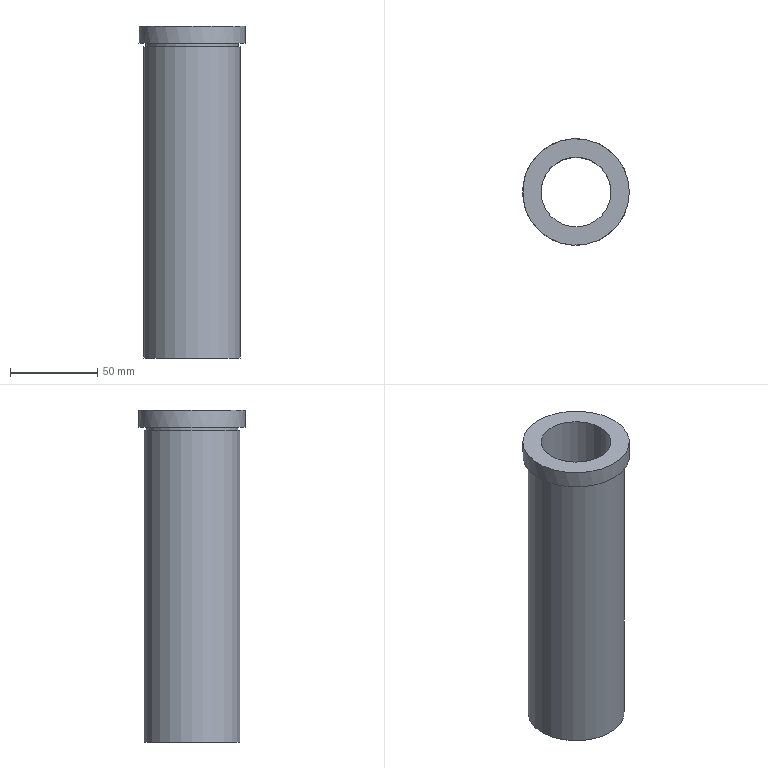Part | STEP file | 车灯-后视镜_id62_x_t | 1 solid | 8 faces | box 61 x 61 x 190 mm | volume 217774 mm3 | plane 4 | cylinder 4 | commonest cylinder face diameters 40 x1 53 x1 55 x1 61 x1
STEP:
#1=CARTESIAN_POINT('',(176.5,-230.,180.5));
#2=VERTEX_POINT('',#1);
#3=CARTESIAN_POINT('',(207.,-230.,180.5));
#4=DIRECTION('',(0.,0.,1.));
#5=DIRECTION('',(-1.,0.,0.));
#6=AXIS2_PLACEMENT_3D('',#3,#4,#5);
#7=CIRCLE('',#6,30.5);
#8=EDGE_CURVE('',#2,#2,#7,.T.);
#9=ORIENTED_EDGE('',*,*,#8,.F.);
#10=EDGE_LOOP('',(#9));
#11=FACE_BOUND('',#10,.T.);
#12=CARTESIAN_POINT('',(233.5,-230.,180.5));
#13=VERTEX_POINT('',#12);
#14=CARTESIAN_POINT('',(207.,-230.,180.5));
#15=DIRECTION('',(0.,0.,-1.));
#16=DIRECTION('',(1.,0.,0.));
#17=AXIS2_PLACEMENT_3D('',#14,#15,#16);
#18=CIRCLE('',#17,26.5);
#19=EDGE_CURVE('',#13,#13,#18,.T.);
#20=ORIENTED_EDGE('',*,*,#19,.F.);
#21=EDGE_LOOP('',(#20));
#22=FACE_BOUND('',#21,.T.);
#23=CARTESIAN_POINT('',(207.,-230.,180.5));
#24=DIRECTION('',(0.,0.,-1.));
#25=DIRECTION('',(1.,0.,0.));
#26=AXIS2_PLACEMENT_3D('',#23,#24,#25);
#27=PLANE('',#26);
#28=ADVANCED_FACE('',(#11,#22),#27,.T.);
#29=CARTESIAN_POINT('',(227.,-230.,190.5));
#30=VERTEX_POINT('',#29);
#31=CARTESIAN_POINT('',(207.,-230.,190.5));
#32=DIRECTION('',(0.,0.,1.));
#33=DIRECTION('',(1.,0.,0.));
#34=AXIS2_PLACEMENT_3D('',#31,#32,#33);
#35=CIRCLE('',#34,20.);
#36=EDGE_CURVE('',#30,#30,#35,.T.);
#37=ORIENTED_EDGE('',*,*,#36,.F.);
#38=EDGE_LOOP('',(#37));
#39=FACE_BOUND('',#38,.T.);
#40=CARTESIAN_POINT('',(237.5,-230.,190.5));
#41=VERTEX_POINT('',#40);
#42=CARTESIAN_POINT('',(207.,-230.,190.5));
#43=DIRECTION('',(0.,0.,-1.));
#44=DIRECTION('',(1.,0.,0.));
#45=AXIS2_PLACEMENT_3D('',#42,#43,#44);
#46=CIRCLE('',#45,30.5);
#47=EDGE_CURVE('',#41,#41,#46,.T.);
#48=ORIENTED_EDGE('',*,*,#47,.F.);
#49=EDGE_LOOP('',(#48));
#50=FACE_BOUND('',#49,.T.);
#51=CARTESIAN_POINT('',(207.,-230.,190.5));
#52=DIRECTION('',(0.,0.,1.));
#53=DIRECTION('',(-1.,0.,0.));
#54=AXIS2_PLACEMENT_3D('',#51,#52,#53);
#55=PLANE('',#54);
#56=ADVANCED_FACE('',(#39,#50),#55,.T.);
#57=ORIENTED_EDGE('',*,*,#8,.T.);
#58=EDGE_LOOP('',(#57));
#59=FACE_BOUND('',#58,.T.);
#60=ORIENTED_EDGE('',*,*,#47,.T.);
#61=EDGE_LOOP('',(#60));
#62=FACE_BOUND('',#61,.T.);
#63=CARTESIAN_POINT('',(207.,-230.,190.5));
#64=DIRECTION('',(0.,0.,-1.));
#65=DIRECTION('',(1.,0.,0.));
#66=AXIS2_PLACEMENT_3D('',#63,#64,#65);
#67=CYLINDRICAL_SURFACE('',#66,30.5);
#68=ADVANCED_FACE('',(#59,#62),#67,.T.);
#69=CARTESIAN_POINT('',(234.5,-230.,0.5));
#70=VERTEX_POINT('',#69);
#71=CARTESIAN_POINT('',(207.,-230.,0.5));
#72=DIRECTION('',(0.,0.,1.));
#73=DIRECTION('',(1.,0.,0.));
#74=AXIS2_PLACEMENT_3D('',#71,#72,#73);
#75=CIRCLE('',#74,27.5);
#76=EDGE_CURVE('',#70,#70,#75,.T.);
#77=ORIENTED_EDGE('',*,*,#76,.T.);
#78=EDGE_LOOP('',(#77));
#79=FACE_BOUND('',#78,.T.);
#80=CARTESIAN_POINT('',(179.5,-230.,178.5));
#81=VERTEX_POINT('',#80);
#82=CARTESIAN_POINT('',(207.,-230.,178.5));
#83=DIRECTION('',(0.,0.,1.));
#84=DIRECTION('',(-1.,0.,0.));
#85=AXIS2_PLACEMENT_3D('',#82,#83,#84);
#86=CIRCLE('',#85,27.5);
#87=EDGE_CURVE('',#81,#81,#86,.T.);
#88=ORIENTED_EDGE('',*,*,#87,.F.);
#89=EDGE_LOOP('',(#88));
#90=FACE_BOUND('',#89,.T.);
#91=CARTESIAN_POINT('',(207.,-230.,60.5));
#92=DIRECTION('',(0.,0.,-1.));
#93=DIRECTION('',(1.,0.,0.));
#94=AXIS2_PLACEMENT_3D('',#91,#92,#93);
#95=CYLINDRICAL_SURFACE('',#94,27.5);
#96=ADVANCED_FACE('',(#79,#90),#95,.T.);
#97=CARTESIAN_POINT('',(227.,-230.,0.5));
#98=VERTEX_POINT('',#97);
#99=CARTESIAN_POINT('',(207.,-230.,0.5));
#100=DIRECTION('',(0.,0.,1.));
#101=DIRECTION('',(1.,0.,0.));
#102=AXIS2_PLACEMENT_3D('',#99,#100,#101);
#103=CIRCLE('',#102,20.);
#104=EDGE_CURVE('',#98,#98,#103,.T.);
#105=ORIENTED_EDGE('',*,*,#104,.F.);
#106=EDGE_LOOP('',(#105));
#107=FACE_BOUND('',#106,.T.);
#108=ORIENTED_EDGE('',*,*,#36,.T.);
#109=EDGE_LOOP('',(#108));
#110=FACE_BOUND('',#109,.T.);
#111=CARTESIAN_POINT('',(207.,-230.,-25.5));
#112=DIRECTION('',(0.,0.,1.));
#113=DIRECTION('',(-1.,0.,0.));
#114=AXIS2_PLACEMENT_3D('',#111,#112,#113);
#115=CYLINDRICAL_SURFACE('',#114,20.);
#116=ADVANCED_FACE('',(#107,#110),#115,.F.);
#117=CARTESIAN_POINT('',(233.5,-230.,178.5));
#118=VERTEX_POINT('',#117);
#119=CARTESIAN_POINT('',(207.,-230.,178.5));
#120=DIRECTION('',(0.,0.,-1.));
#121=DIRECTION('',(1.,0.,0.));
#122=AXIS2_PLACEMENT_3D('',#119,#120,#121);
#123=CIRCLE('',#122,26.5);
#124=EDGE_CURVE('',#118,#118,#123,.T.);
#125=ORIENTED_EDGE('',*,*,#124,.F.);
#126=EDGE_LOOP('',(#125));
#127=FACE_BOUND('',#126,.T.);
#128=ORIENTED_EDGE('',*,*,#19,.T.);
#129=EDGE_LOOP('',(#128));
#130=FACE_BOUND('',#129,.T.);
#131=CARTESIAN_POINT('',(207.,-230.,179.5));
#132=DIRECTION('',(0.,0.,-1.));
#133=DIRECTION('',(1.,0.,0.));
#134=AXIS2_PLACEMENT_3D('',#131,#132,#133);
#135=CYLINDRICAL_SURFACE('',#134,26.5);
#136=ADVANCED_FACE('',(#127,#130),#135,.T.);
#137=ORIENTED_EDGE('',*,*,#87,.T.);
#138=EDGE_LOOP('',(#137));
#139=FACE_BOUND('',#138,.T.);
#140=ORIENTED_EDGE('',*,*,#124,.T.);
#141=EDGE_LOOP('',(#140));
#142=FACE_BOUND('',#141,.T.);
#143=CARTESIAN_POINT('',(207.,-230.,178.5));
#144=DIRECTION('',(0.,0.,-1.));
#145=DIRECTION('',(1.,0.,0.));
#146=AXIS2_PLACEMENT_3D('',#143,#144,#145);
#147=PLANE('',#146);
#148=ADVANCED_FACE('',(#139,#142),#147,.F.);
#149=ORIENTED_EDGE('',*,*,#76,.F.);
#150=EDGE_LOOP('',(#149));
#151=FACE_BOUND('',#150,.T.);
#152=ORIENTED_EDGE('',*,*,#104,.T.);
#153=EDGE_LOOP('',(#152));
#154=FACE_BOUND('',#153,.T.);
#155=CARTESIAN_POINT('',(250.,-273.,0.5));
#156=DIRECTION('',(0.,0.,1.));
#157=DIRECTION('',(1.,0.,0.));
#158=AXIS2_PLACEMENT_3D('',#155,#156,#157);
#159=PLANE('',#158);
#160=ADVANCED_FACE('',(#151,#154),#159,.F.);
#161=CLOSED_SHELL('',(#28,#56,#68,#96,#116,#136,#148,#160));
#162=MANIFOLD_SOLID_BREP('',#161);
#163=(LENGTH_UNIT()NAMED_UNIT(*)SI_UNIT(.MILLI.,.METRE.));
#164=UNCERTAINTY_MEASURE_WITH_UNIT(LENGTH_MEASURE(0.00002),#163,'','');
#165=(NAMED_UNIT(*)PLANE_ANGLE_UNIT()SI_UNIT($,.RADIAN.));
#166=PLANE_ANGLE_MEASURE_WITH_UNIT(PLANE_ANGLE_MEASURE(0.01745),#165);
#167=DIMENSIONAL_EXPONENTS(0.,0.,0.,0.,0.,0.,0.);
#168=(CONVERSION_BASED_UNIT('DEGREE',#166)NAMED_UNIT(#167)PLANE_ANGLE_UNIT());
#169=(NAMED_UNIT(*)SI_UNIT($,.STERADIAN.)SOLID_ANGLE_UNIT());
#170=(GEOMETRIC_REPRESENTATION_CONTEXT(3)GLOBAL_UNCERTAINTY_ASSIGNED_CONTEXT((#164))GLOBAL_UNIT_ASSIGNED_CONTEXT((#163,#168,#169))REPRESENTATION_CONTEXT('',''));
#171=ADVANCED_BREP_SHAPE_REPRESENTATION('',(#162),#170);